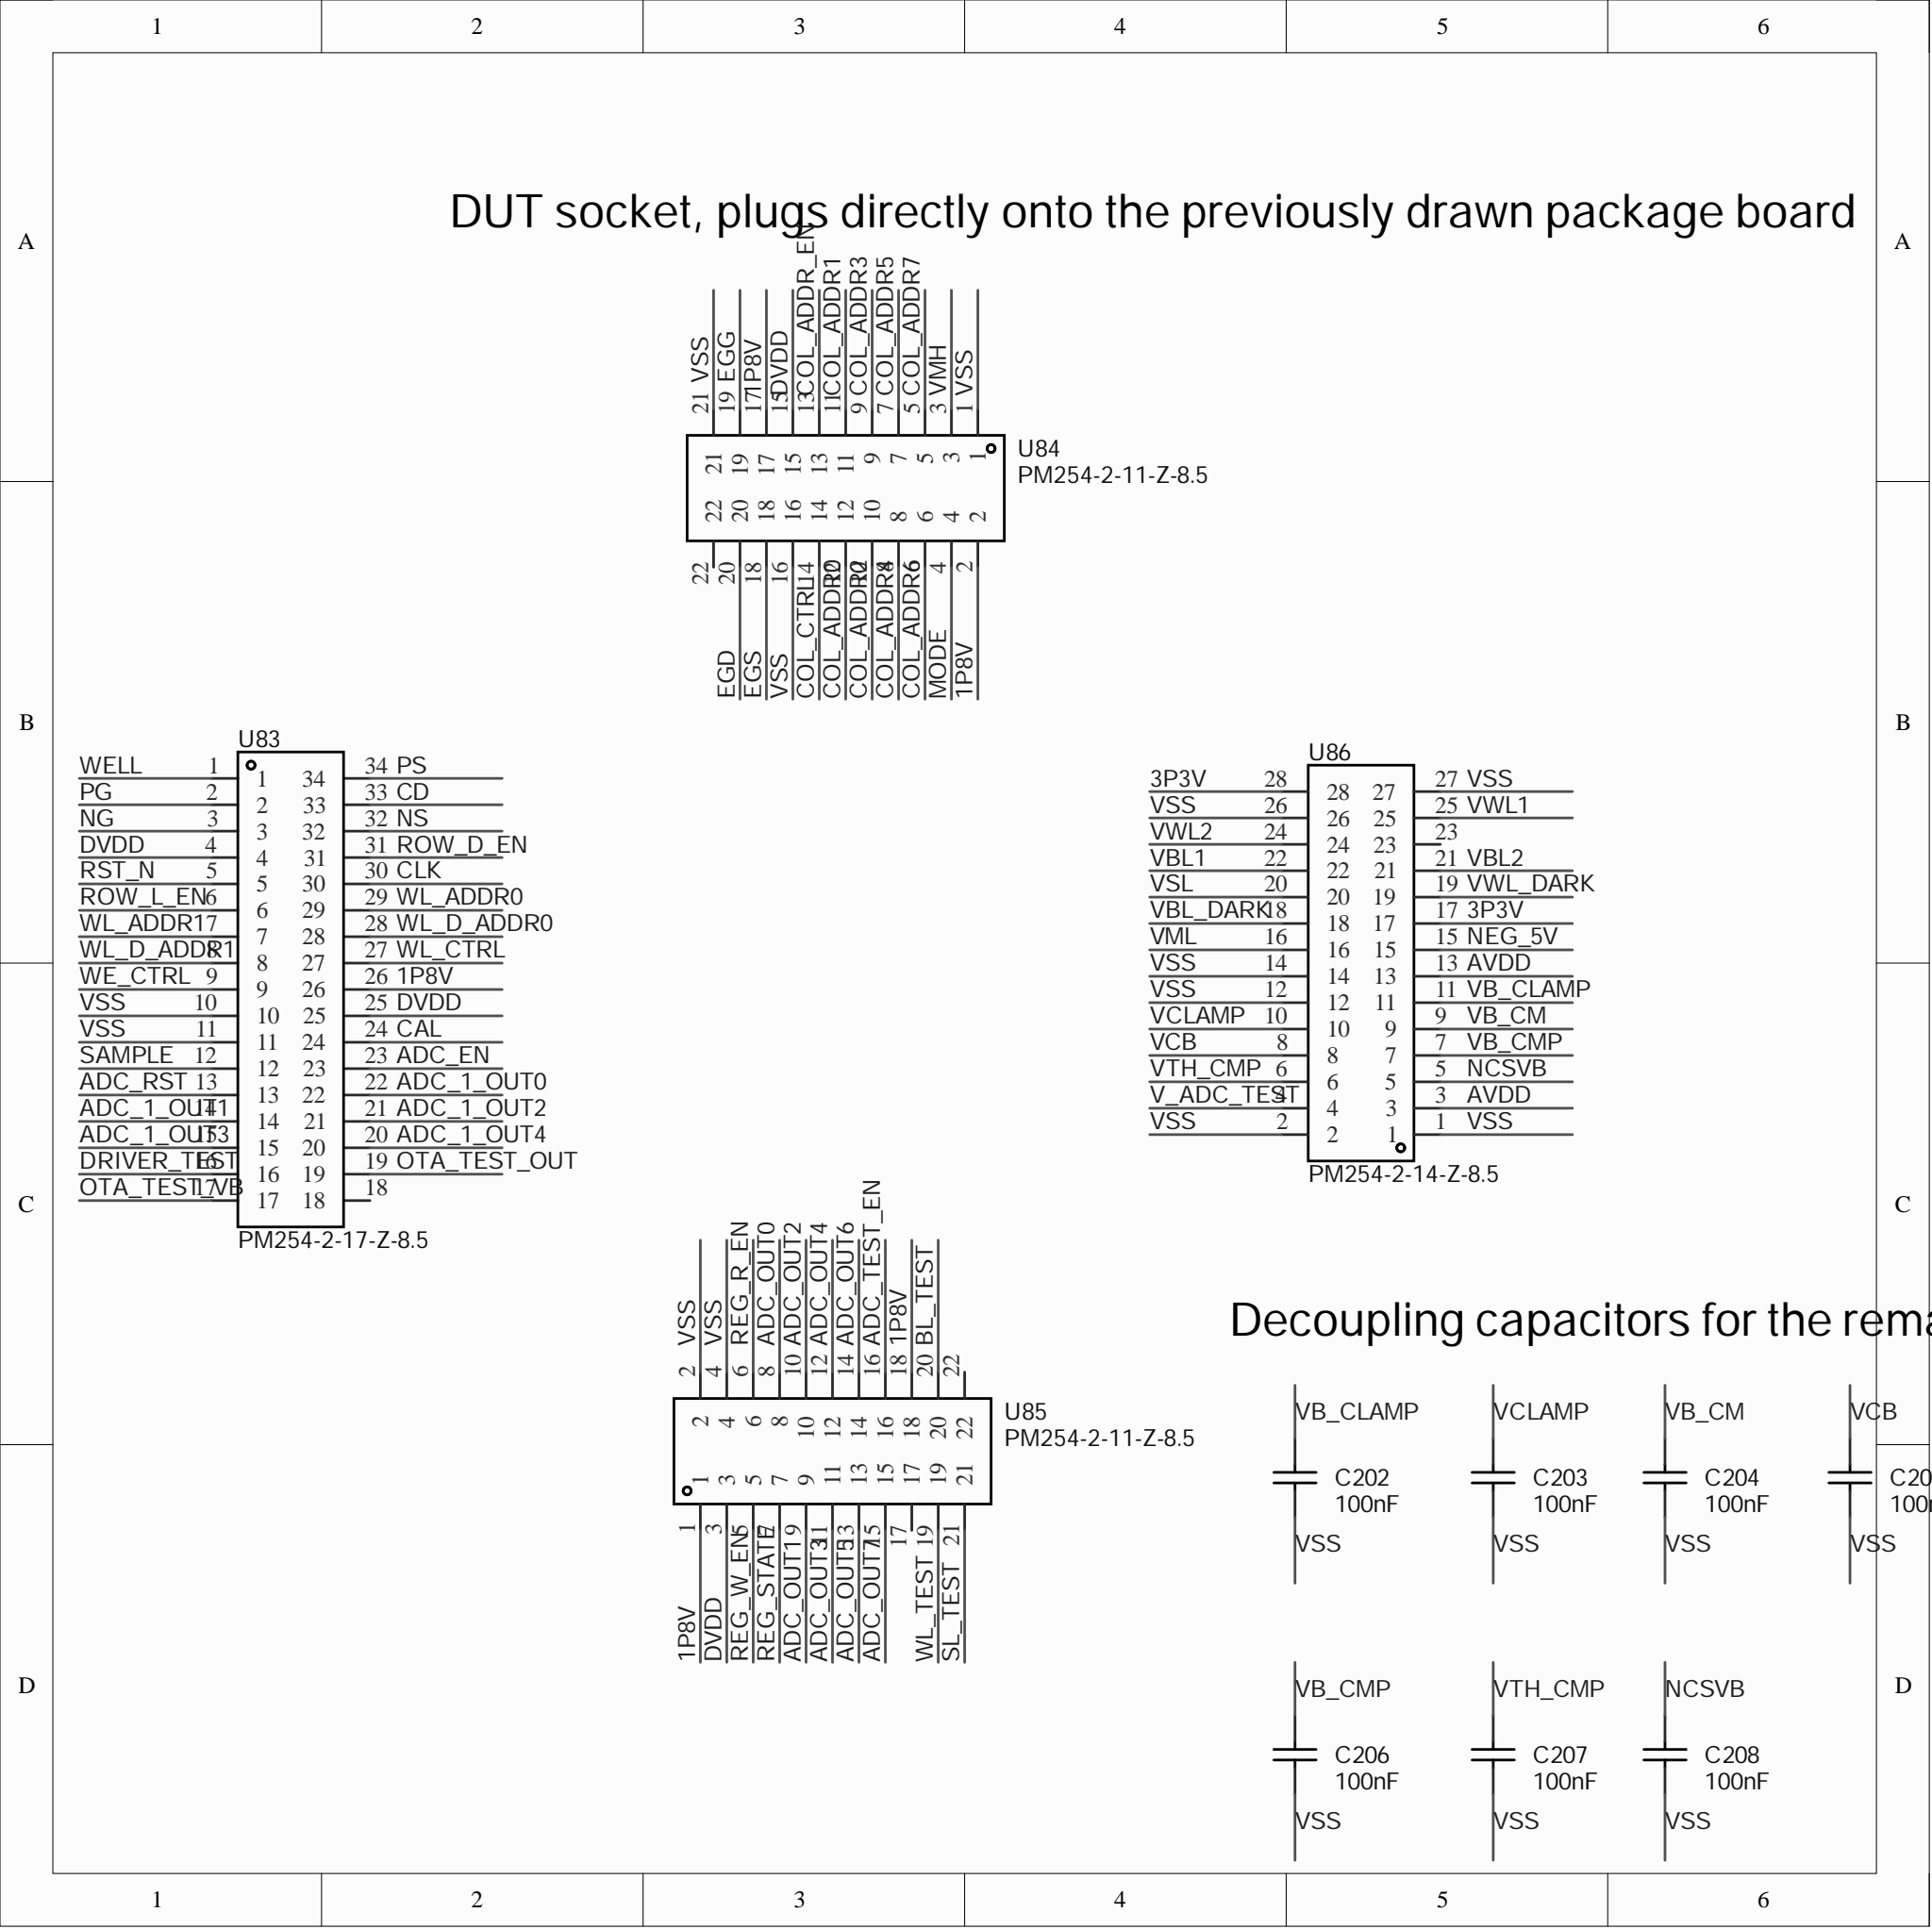Circuit board | Altium Designer | 201 parts | 197 nets | one sheet of the schematic
Parts on this sheet (reference | value | footprint):
C202 | 100nF | C0402
C203 | 100nF | C0402
C204 | 100nF | C0402
C205 | 100nF | C0402
C206 | 100nF | C0402
C207 | 100nF | C0402
C208 | 100nF | C0402
U83 | PM254-2-17-Z-8.5 | HDR-TH_34P-P2.54-V-F-R2-C17-S2.54-1
U84 | PM254-2-11-Z-8.5 | HDR-TH_22P-P2.54-V-F-R2-C11-S2.54
U85 | PM254-2-11-Z-8.5 | HDR-TH_22P-P2.54-V-F-R2-C11-S2.54
U86 | PM254-2-14-Z-8.5 | HDR-TH_28P-P2.54-V-F-R2-C14-S2.54-1
Nets of these parts (net: part-pin ...):
WL_TEST: U85-19
WL_D_ADDR1: U83-8
WL_D_ADDR0: U83-28
WL_CTRL: U83-27
WL_ADDR1: U83-7
WL_ADDR0: U83-29
WELL: U83-1
WE_CTRL: U83-9
VWL_DARK: U86-19
VWL2: U86-24
VWL1: U86-25
VTH_CMP: C207-1 U86-6
VSS: C202-2 C203-2 C204-2 C205-2 C206-2 C207-2 C208-2 U85-2 U85-4 U83-10 U83-11 U84-1 U84-16 U84-21 U86-1 U86-2 U86-12 U86-14 U86-26 U86-27
VSL: U86-20
VML: U86-16
VMH: U84-3
VCLAMP: C203-1 U86-10
VCB: C205-1 U86-8
VBL_DARK: U86-18
VBL2: U86-21
VBL1: U86-22
VB_CMP: C206-1 U86-7
VB_CM: C204-1 U86-9
VB_CLAMP: C202-1 U86-11
V_ADC_TEST: U86-4
SL_TEST: U85-21
SAMPLE: U83-12
RST_N: U83-5
ROW_L_EN: U83-6
ROW_D_EN: U83-31
REG_W_EN: U85-5
REG_STATE: U85-7
REG_R_EN: U85-6
PS: U83-34
PG: U83-2
OTA_TEST_VB: U83-17
OTA_TEST_OUT: U83-19
NS: U83-32
NG: U83-3
NEG_5V: U86-15
NCSVB: C208-1 U86-5
MODE: U84-4
EGS: U84-18
EGG: U84-19
EGD: U84-20
DVDD: U85-3 U83-4 U83-25 U84-15
DRIVER_TEST: U83-16
COL_CTRL: U84-14
COL_ADDR_EN: U84-13
COL_ADDR7: U84-5
COL_ADDR6: U84-6
COL_ADDR5: U84-7
COL_ADDR4: U84-8
COL_ADDR3: U84-9
COL_ADDR2: U84-10
COL_ADDR1: U84-11
COL_ADDR0: U84-12
CLK: U83-30
CD: U83-33
CAL: U83-24
BL_TEST: U85-20
AVDD: U86-3 U86-13
ADC_TEST_EN: U85-16
ADC_RST: U83-13
ADC_OUT7: U85-15
ADC_OUT6: U85-14
ADC_OUT5: U85-13
ADC_OUT4: U85-12
ADC_OUT3: U85-11
ADC_OUT2: U85-10
ADC_OUT1: U85-9
ADC_OUT0: U85-8
ADC_EN: U83-23
ADC_1_OUT4: U83-20
ADC_1_OUT3: U83-15
ADC_1_OUT2: U83-21
ADC_1_OUT1: U83-14
ADC_1_OUT0: U83-22
3P3V: U86-17 U86-28
1P8V: U85-1 U85-18 U83-26 U84-2 U84-17